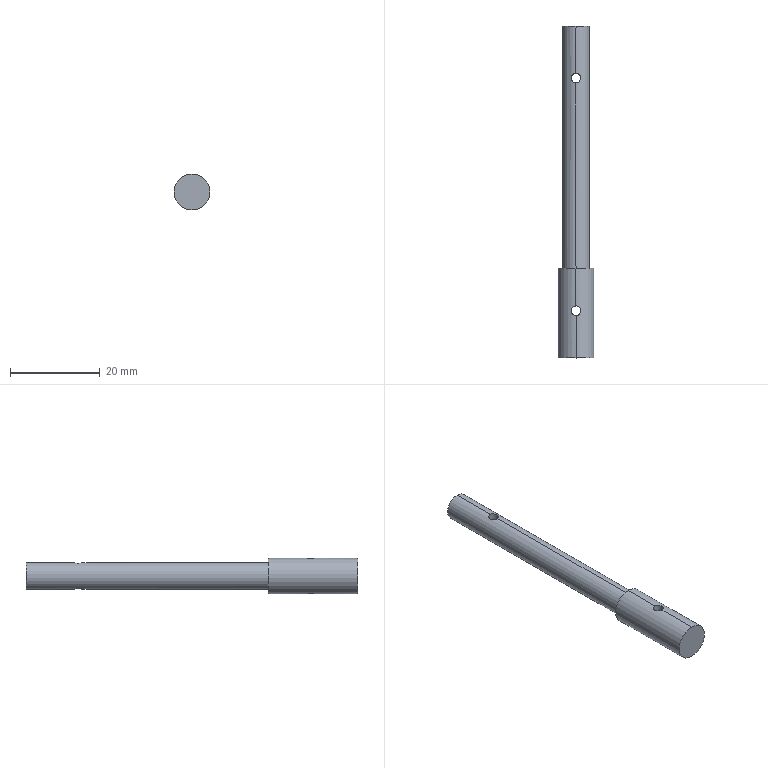Part | SolidWorks | features ICE 1, Revolution 1 | 1 solid | 11 faces | box 8 x 74 x 8 mm | volume 2480 mm3 | cylinder 8 | plane 3 | commonest cylinder face diameters 2.2 x4 6 x2 8 x2
STEP:
#1=CARTESIAN_POINT('',(0.,55.397,-3.));
#2=VERTEX_POINT('',#1);
#3=CARTESIAN_POINT('',(-1.1,56.497,-2.791));
#4=VERTEX_POINT('',#3);
#5=CARTESIAN_POINT('',(0.,55.397,-3.));
#6=CARTESIAN_POINT('',(-0.1445,55.397,-3.));
#7=CARTESIAN_POINT('',(-0.2902,55.427,-2.989));
#8=CARTESIAN_POINT('',(-0.556,55.537,-2.951));
#9=CARTESIAN_POINT('',(-0.6765,55.618,-2.925));
#10=CARTESIAN_POINT('',(-0.8798,55.822,-2.87));
#11=CARTESIAN_POINT('',(-0.9601,55.941,-2.843));
#12=CARTESIAN_POINT('',(-1.043,56.141,-2.813));
#13=CARTESIAN_POINT('',(-1.064,56.21,-2.805));
#14=CARTESIAN_POINT('',(-1.093,56.351,-2.794));
#15=CARTESIAN_POINT('',(-1.1,56.425,-2.791));
#16=CARTESIAN_POINT('',(-1.1,56.497,-2.791));
#17=B_SPLINE_CURVE_WITH_KNOTS('',3,(#5,#6,#7,#8,#9,#10,#11,#12,#13,#14,#15,#16),.UNSPECIFIED.,.F.,.F.,(4,2,2,2,2,4),(0.00347,0.003903,0.004337,0.00477,0.004987,0.005204),.UNSPECIFIED.);
#18=EDGE_CURVE('',#2,#4,#17,.T.);
#19=ORIENTED_EDGE('',*,*,#18,.T.);
#20=CARTESIAN_POINT('',(-1.1,56.497,2.791));
#21=VERTEX_POINT('',#20);
#22=CARTESIAN_POINT('',(-1.1,56.497,-15.));
#23=DIRECTION('',(0.,0.,1.));
#24=VECTOR('',#23,1000.);
#25=LINE('',#22,#24);
#26=EDGE_CURVE('',#4,#21,#25,.T.);
#27=ORIENTED_EDGE('',*,*,#26,.T.);
#28=CARTESIAN_POINT('',(0.,55.397,3.));
#29=VERTEX_POINT('',#28);
#30=CARTESIAN_POINT('',(-1.1,56.497,2.791));
#31=CARTESIAN_POINT('',(-1.1,56.353,2.791));
#32=CARTESIAN_POINT('',(-1.071,56.207,2.803));
#33=CARTESIAN_POINT('',(-0.9601,55.942,2.843));
#34=CARTESIAN_POINT('',(-0.8795,55.821,2.87));
#35=CARTESIAN_POINT('',(-0.6761,55.618,2.925));
#36=CARTESIAN_POINT('',(-0.5563,55.537,2.951));
#37=CARTESIAN_POINT('',(-0.3563,55.454,2.98));
#38=CARTESIAN_POINT('',(-0.2876,55.433,2.987));
#39=CARTESIAN_POINT('',(-0.1461,55.405,2.997));
#40=CARTESIAN_POINT('',(-0.07247,55.397,3.));
#41=CARTESIAN_POINT('',(0.,55.397,3.));
#42=B_SPLINE_CURVE_WITH_KNOTS('',3,(#30,#31,#32,#33,#34,#35,#36,#37,#38,#39,#40,#41),.UNSPECIFIED.,.F.,.F.,(4,2,2,2,2,4),(0.00347,0.003903,0.004336,0.00477,0.004987,0.005203),.UNSPECIFIED.);
#43=EDGE_CURVE('',#21,#29,#42,.T.);
#44=ORIENTED_EDGE('',*,*,#43,.T.);
#45=CARTESIAN_POINT('',(1.1,56.497,2.791));
#46=VERTEX_POINT('',#45);
#47=CARTESIAN_POINT('',(0.,55.397,3.));
#48=CARTESIAN_POINT('',(0.145,55.397,3.));
#49=CARTESIAN_POINT('',(0.2907,55.427,2.989));
#50=CARTESIAN_POINT('',(0.5558,55.537,2.951));
#51=CARTESIAN_POINT('',(0.6773,55.619,2.924));
#52=CARTESIAN_POINT('',(0.879,55.821,2.87));
#53=CARTESIAN_POINT('',(0.9599,55.941,2.843));
#54=CARTESIAN_POINT('',(1.071,56.208,2.803));
#55=CARTESIAN_POINT('',(1.1,56.351,2.791));
#56=CARTESIAN_POINT('',(1.1,56.497,2.791));
#57=B_SPLINE_CURVE_WITH_KNOTS('',3,(#47,#48,#49,#50,#51,#52,#53,#54,#55,#56),.UNSPECIFIED.,.F.,.F.,(4,2,2,2,4),(0.005203,0.005637,0.006071,0.006505,0.006938),.UNSPECIFIED.);
#58=EDGE_CURVE('',#29,#46,#57,.T.);
#59=ORIENTED_EDGE('',*,*,#58,.T.);
#60=CARTESIAN_POINT('',(1.1,56.497,-2.791));
#61=VERTEX_POINT('',#60);
#62=CARTESIAN_POINT('',(1.1,56.497,-15.));
#63=DIRECTION('',(0.,0.,1.));
#64=VECTOR('',#63,1000.);
#65=LINE('',#62,#64);
#66=EDGE_CURVE('',#61,#46,#65,.T.);
#67=ORIENTED_EDGE('',*,*,#66,.F.);
#68=CARTESIAN_POINT('',(1.1,56.497,-2.791));
#69=CARTESIAN_POINT('',(1.1,56.352,-2.791));
#70=CARTESIAN_POINT('',(1.071,56.208,-2.803));
#71=CARTESIAN_POINT('',(0.9594,55.94,-2.843));
#72=CARTESIAN_POINT('',(0.8783,55.82,-2.87));
#73=CARTESIAN_POINT('',(0.6763,55.618,-2.925));
#74=CARTESIAN_POINT('',(0.555,55.537,-2.951));
#75=CARTESIAN_POINT('',(0.2904,55.427,-2.989));
#76=CARTESIAN_POINT('',(0.1445,55.397,-3.));
#77=CARTESIAN_POINT('',(0.,55.397,-3.));
#78=B_SPLINE_CURVE_WITH_KNOTS('',3,(#68,#69,#70,#71,#72,#73,#74,#75,#76,#77),.UNSPECIFIED.,.F.,.F.,(4,2,2,2,4),(0.001735,0.002169,0.002603,0.003036,0.00347),.UNSPECIFIED.);
#79=EDGE_CURVE('',#61,#2,#78,.T.);
#80=ORIENTED_EDGE('',*,*,#79,.T.);
#81=EDGE_LOOP('',(#19,#27,#44,#59,#67,#80));
#82=FACE_OUTER_BOUND('',#81,.T.);
#83=CARTESIAN_POINT('',(0.,56.497,-15.));
#84=DIRECTION('',(0.,0.,1.));
#85=DIRECTION('',(1.,0.,0.));
#86=AXIS2_PLACEMENT_3D('',#83,#84,#85);
#87=CYLINDRICAL_SURFACE('',#86,1.1);
#88=ADVANCED_FACE('',(#82),#87,.F.);
#89=CARTESIAN_POINT('',(0.,3.497,-4.));
#90=VERTEX_POINT('',#89);
#91=CARTESIAN_POINT('',(-1.1,4.597,-3.846));
#92=VERTEX_POINT('',#91);
#93=CARTESIAN_POINT('',(0.,3.497,-4.));
#94=CARTESIAN_POINT('',(-0.144,3.497,-4.));
#95=CARTESIAN_POINT('',(-0.2894,3.526,-3.992));
#96=CARTESIAN_POINT('',(-0.5545,3.637,-3.964));
#97=CARTESIAN_POINT('',(-0.6762,3.718,-3.944));
#98=CARTESIAN_POINT('',(-0.8792,3.921,-3.904));
#99=CARTESIAN_POINT('',(-0.96,4.041,-3.884));
#100=CARTESIAN_POINT('',(-1.071,4.309,-3.854));
#101=CARTESIAN_POINT('',(-1.1,4.452,-3.846));
#102=CARTESIAN_POINT('',(-1.1,4.597,-3.846));
#103=B_SPLINE_CURVE_WITH_KNOTS('',3,(#93,#94,#95,#96,#97,#98,#99,#100,#101,#102),.UNSPECIFIED.,.F.,.F.,(4,2,2,2,4),(0.003456,0.003888,0.00432,0.004752,0.005183),.UNSPECIFIED.);
#104=EDGE_CURVE('',#90,#92,#103,.T.);
#105=ORIENTED_EDGE('',*,*,#104,.T.);
#106=CARTESIAN_POINT('',(-1.1,4.597,3.846));
#107=VERTEX_POINT('',#106);
#108=CARTESIAN_POINT('',(-1.1,4.597,-15.));
#109=DIRECTION('',(0.,0.,1.));
#110=VECTOR('',#109,1000.);
#111=LINE('',#108,#110);
#112=EDGE_CURVE('',#92,#107,#111,.T.);
#113=ORIENTED_EDGE('',*,*,#112,.T.);
#114=CARTESIAN_POINT('',(0.,3.497,4.));
#115=VERTEX_POINT('',#114);
#116=CARTESIAN_POINT('',(-1.1,4.597,3.846));
#117=CARTESIAN_POINT('',(-1.1,4.453,3.846));
#118=CARTESIAN_POINT('',(-1.071,4.308,3.854));
#119=CARTESIAN_POINT('',(-0.9608,4.043,3.883));
#120=CARTESIAN_POINT('',(-0.8795,3.921,3.903));
#121=CARTESIAN_POINT('',(-0.6766,3.718,3.944));
#122=CARTESIAN_POINT('',(-0.5564,3.637,3.963));
#123=CARTESIAN_POINT('',(-0.2883,3.526,3.992));
#124=CARTESIAN_POINT('',(-0.1451,3.497,4.));
#125=CARTESIAN_POINT('',(0.,3.497,4.));
#126=B_SPLINE_CURVE_WITH_KNOTS('',3,(#116,#117,#118,#119,#120,#121,#122,#123,#124,#125),.UNSPECIFIED.,.F.,.F.,(4,2,2,2,4),(0.003456,0.003888,0.00432,0.004752,0.005183),.UNSPECIFIED.);
#127=EDGE_CURVE('',#107,#115,#126,.T.);
#128=ORIENTED_EDGE('',*,*,#127,.T.);
#129=CARTESIAN_POINT('',(1.1,4.597,3.846));
#130=VERTEX_POINT('',#129);
#131=CARTESIAN_POINT('',(0.,3.497,4.));
#132=CARTESIAN_POINT('',(0.145,3.497,4.));
#133=CARTESIAN_POINT('',(0.2895,3.527,3.992));
#134=CARTESIAN_POINT('',(0.5547,3.637,3.964));
#135=CARTESIAN_POINT('',(0.6767,3.719,3.944));
#136=CARTESIAN_POINT('',(0.8785,3.92,3.904));
#137=CARTESIAN_POINT('',(0.9603,4.042,3.883));
#138=CARTESIAN_POINT('',(1.071,4.307,3.854));
#139=CARTESIAN_POINT('',(1.1,4.451,3.846));
#140=CARTESIAN_POINT('',(1.1,4.597,3.846));
#141=B_SPLINE_CURVE_WITH_KNOTS('',3,(#131,#132,#133,#134,#135,#136,#137,#138,#139,#140),.UNSPECIFIED.,.F.,.F.,(4,2,2,2,4),(0.005183,0.005615,0.006047,0.006479,0.006911),.UNSPECIFIED.);
#142=EDGE_CURVE('',#115,#130,#141,.T.);
#143=ORIENTED_EDGE('',*,*,#142,.T.);
#144=CARTESIAN_POINT('',(1.1,4.597,-3.846));
#145=VERTEX_POINT('',#144);
#146=CARTESIAN_POINT('',(1.1,4.597,-15.));
#147=DIRECTION('',(0.,0.,1.));
#148=VECTOR('',#147,1000.);
#149=LINE('',#146,#148);
#150=EDGE_CURVE('',#145,#130,#149,.T.);
#151=ORIENTED_EDGE('',*,*,#150,.F.);
#152=CARTESIAN_POINT('',(1.1,4.597,-3.846));
#153=CARTESIAN_POINT('',(1.1,4.453,-3.846));
#154=CARTESIAN_POINT('',(1.071,4.309,-3.854));
#155=CARTESIAN_POINT('',(0.9602,4.042,-3.883));
#156=CARTESIAN_POINT('',(0.8792,3.921,-3.904));
#157=CARTESIAN_POINT('',(0.6757,3.718,-3.944));
#158=CARTESIAN_POINT('',(0.5544,3.637,-3.964));
#159=CARTESIAN_POINT('',(0.2891,3.526,-3.992));
#160=CARTESIAN_POINT('',(0.144,3.497,-4.));
#161=CARTESIAN_POINT('',(0.,3.497,-4.));
#162=B_SPLINE_CURVE_WITH_KNOTS('',3,(#152,#153,#154,#155,#156,#157,#158,#159,#160,#161),.UNSPECIFIED.,.F.,.F.,(4,2,2,2,4),(0.001728,0.00216,0.002592,0.003024,0.003456),.UNSPECIFIED.);
#163=EDGE_CURVE('',#145,#90,#162,.T.);
#164=ORIENTED_EDGE('',*,*,#163,.T.);
#165=EDGE_LOOP('',(#105,#113,#128,#143,#151,#164));
#166=FACE_OUTER_BOUND('',#165,.T.);
#167=CARTESIAN_POINT('',(0.,4.597,-15.));
#168=DIRECTION('',(0.,0.,1.));
#169=DIRECTION('',(1.,0.,0.));
#170=AXIS2_PLACEMENT_3D('',#167,#168,#169);
#171=CYLINDRICAL_SURFACE('',#170,1.1);
#172=ADVANCED_FACE('',(#166),#171,.F.);
#173=CARTESIAN_POINT('',(0.,14.097,-4.));
#174=VERTEX_POINT('',#173);
#175=CARTESIAN_POINT('',(0.,14.097,4.));
#176=VERTEX_POINT('',#175);
#177=CARTESIAN_POINT('',(0.,14.097,0.));
#178=DIRECTION('',(0.,-1.,0.));
#179=DIRECTION('',(0.,0.,-1.));
#180=AXIS2_PLACEMENT_3D('',#177,#178,#179);
#181=CIRCLE('',#180,4.);
#182=EDGE_CURVE('',#174,#176,#181,.T.);
#183=ORIENTED_EDGE('',*,*,#182,.T.);
#184=CARTESIAN_POINT('',(0.,5.697,4.));
#185=VERTEX_POINT('',#184);
#186=CARTESIAN_POINT('',(0.,0.,4.));
#187=DIRECTION('',(0.,-1.,0.));
#188=VECTOR('',#187,1000.);
#189=LINE('',#186,#188);
#190=EDGE_CURVE('',#176,#185,#189,.T.);
#191=ORIENTED_EDGE('',*,*,#190,.T.);
#192=CARTESIAN_POINT('',(1.1,4.597,3.846));
#193=CARTESIAN_POINT('',(1.1,4.744,3.846));
#194=CARTESIAN_POINT('',(1.071,4.887,3.854));
#195=CARTESIAN_POINT('',(0.9602,5.153,3.883));
#196=CARTESIAN_POINT('',(0.8785,5.275,3.904));
#197=CARTESIAN_POINT('',(0.6765,5.476,3.944));
#198=CARTESIAN_POINT('',(0.5542,5.558,3.964));
#199=CARTESIAN_POINT('',(0.2896,5.668,3.992));
#200=CARTESIAN_POINT('',(0.1443,5.697,4.));
#201=CARTESIAN_POINT('',(0.,5.697,4.));
#202=B_SPLINE_CURVE_WITH_KNOTS('',3,(#192,#193,#194,#195,#196,#197,#198,#199,#200,#201),.UNSPECIFIED.,.F.,.F.,(4,2,2,2,4),(0.,0.0004321,0.0008642,0.001296,0.001728),.UNSPECIFIED.);
#203=EDGE_CURVE('',#130,#185,#202,.T.);
#204=ORIENTED_EDGE('',*,*,#203,.F.);
#205=ORIENTED_EDGE('',*,*,#142,.F.);
#206=CARTESIAN_POINT('',(0.,-5.903,4.));
#207=VERTEX_POINT('',#206);
#208=CARTESIAN_POINT('',(0.,0.,4.));
#209=DIRECTION('',(0.,-1.,0.));
#210=VECTOR('',#209,1000.);
#211=LINE('',#208,#210);
#212=EDGE_CURVE('',#115,#207,#211,.T.);
#213=ORIENTED_EDGE('',*,*,#212,.T.);
#214=CARTESIAN_POINT('',(0.,-5.903,-4.));
#215=VERTEX_POINT('',#214);
#216=CARTESIAN_POINT('',(0.,-5.903,0.));
#217=DIRECTION('',(0.,-1.,0.));
#218=DIRECTION('',(0.,0.,-1.));
#219=AXIS2_PLACEMENT_3D('',#216,#217,#218);
#220=CIRCLE('',#219,4.);
#221=EDGE_CURVE('',#215,#207,#220,.T.);
#222=ORIENTED_EDGE('',*,*,#221,.F.);
#223=CARTESIAN_POINT('',(0.,0.,-4.));
#224=DIRECTION('',(0.,-1.,0.));
#225=VECTOR('',#224,1000.);
#226=LINE('',#223,#225);
#227=EDGE_CURVE('',#90,#215,#226,.T.);
#228=ORIENTED_EDGE('',*,*,#227,.F.);
#229=ORIENTED_EDGE('',*,*,#163,.F.);
#230=CARTESIAN_POINT('',(0.,5.697,-4.));
#231=VERTEX_POINT('',#230);
#232=CARTESIAN_POINT('',(0.,5.697,-4.));
#233=CARTESIAN_POINT('',(0.1462,5.697,-4.));
#234=CARTESIAN_POINT('',(0.2895,5.668,-3.992));
#235=CARTESIAN_POINT('',(0.5557,5.558,-3.963));
#236=CARTESIAN_POINT('',(0.6773,5.476,-3.944));
#237=CARTESIAN_POINT('',(0.8792,5.274,-3.904));
#238=CARTESIAN_POINT('',(0.9609,5.152,-3.883));
#239=CARTESIAN_POINT('',(1.071,4.887,-3.854));
#240=CARTESIAN_POINT('',(1.1,4.742,-3.846));
#241=CARTESIAN_POINT('',(1.1,4.597,-3.846));
#242=B_SPLINE_CURVE_WITH_KNOTS('',3,(#232,#233,#234,#235,#236,#237,#238,#239,#240,#241),.UNSPECIFIED.,.F.,.F.,(4,2,2,2,4),(0.,0.0004321,0.0008642,0.001296,0.001728),.UNSPECIFIED.);
#243=EDGE_CURVE('',#231,#145,#242,.T.);
#244=ORIENTED_EDGE('',*,*,#243,.F.);
#245=CARTESIAN_POINT('',(0.,0.,-4.));
#246=DIRECTION('',(0.,-1.,0.));
#247=VECTOR('',#246,1000.);
#248=LINE('',#245,#247);
#249=EDGE_CURVE('',#174,#231,#248,.T.);
#250=ORIENTED_EDGE('',*,*,#249,.F.);
#251=EDGE_LOOP('',(#183,#191,#204,#205,#213,#222,#228,#229,#244,#250));
#252=FACE_OUTER_BOUND('',#251,.T.);
#253=CARTESIAN_POINT('',(0.,0.,0.));
#254=DIRECTION('',(0.,-1.,0.));
#255=DIRECTION('',(0.,0.,-1.));
#256=AXIS2_PLACEMENT_3D('',#253,#254,#255);
#257=CYLINDRICAL_SURFACE('',#256,4.);
#258=ADVANCED_FACE('',(#252),#257,.T.);
#259=CARTESIAN_POINT('',(0.,68.097,-3.));
#260=VERTEX_POINT('',#259);
#261=CARTESIAN_POINT('',(0.,68.097,3.));
#262=VERTEX_POINT('',#261);
#263=CARTESIAN_POINT('',(0.,68.097,0.));
#264=DIRECTION('',(0.,-1.,0.));
#265=DIRECTION('',(0.,0.,-1.));
#266=AXIS2_PLACEMENT_3D('',#263,#264,#265);
#267=CIRCLE('',#266,3.);
#268=EDGE_CURVE('',#260,#262,#267,.T.);
#269=ORIENTED_EDGE('',*,*,#268,.T.);
#270=CARTESIAN_POINT('',(0.,57.597,3.));
#271=VERTEX_POINT('',#270);
#272=CARTESIAN_POINT('',(0.,0.,3.));
#273=DIRECTION('',(0.,-1.,0.));
#274=VECTOR('',#273,1000.);
#275=LINE('',#272,#274);
#276=EDGE_CURVE('',#262,#271,#275,.T.);
#277=ORIENTED_EDGE('',*,*,#276,.T.);
#278=CARTESIAN_POINT('',(1.1,56.497,2.791));
#279=CARTESIAN_POINT('',(1.1,56.644,2.791));
#280=CARTESIAN_POINT('',(1.071,56.788,2.803));
#281=CARTESIAN_POINT('',(0.9597,57.054,2.843));
#282=CARTESIAN_POINT('',(0.8781,57.175,2.87));
#283=CARTESIAN_POINT('',(0.6769,57.376,2.924));
#284=CARTESIAN_POINT('',(0.5552,57.458,2.951));
#285=CARTESIAN_POINT('',(0.2907,57.568,2.989));
#286=CARTESIAN_POINT('',(0.145,57.597,3.));
#287=CARTESIAN_POINT('',(0.,57.597,3.));
#288=B_SPLINE_CURVE_WITH_KNOTS('',3,(#278,#279,#280,#281,#282,#283,#284,#285,#286,#287),.UNSPECIFIED.,.F.,.F.,(4,2,2,2,4),(0.,0.0004338,0.0008676,0.001301,0.001735),.UNSPECIFIED.);
#289=EDGE_CURVE('',#46,#271,#288,.T.);
#290=ORIENTED_EDGE('',*,*,#289,.F.);
#291=ORIENTED_EDGE('',*,*,#58,.F.);
#292=CARTESIAN_POINT('',(0.,14.097,3.));
#293=VERTEX_POINT('',#292);
#294=CARTESIAN_POINT('',(0.,0.,3.));
#295=DIRECTION('',(0.,-1.,0.));
#296=VECTOR('',#295,1000.);
#297=LINE('',#294,#296);
#298=EDGE_CURVE('',#29,#293,#297,.T.);
#299=ORIENTED_EDGE('',*,*,#298,.T.);
#300=CARTESIAN_POINT('',(0.,14.097,-3.));
#301=VERTEX_POINT('',#300);
#302=CARTESIAN_POINT('',(0.,14.097,0.));
#303=DIRECTION('',(0.,-1.,0.));
#304=DIRECTION('',(0.,0.,-1.));
#305=AXIS2_PLACEMENT_3D('',#302,#303,#304);
#306=CIRCLE('',#305,3.);
#307=EDGE_CURVE('',#301,#293,#306,.T.);
#308=ORIENTED_EDGE('',*,*,#307,.F.);
#309=CARTESIAN_POINT('',(0.,0.,-3.));
#310=DIRECTION('',(0.,-1.,0.));
#311=VECTOR('',#310,1000.);
#312=LINE('',#309,#311);
#313=EDGE_CURVE('',#2,#301,#312,.T.);
#314=ORIENTED_EDGE('',*,*,#313,.F.);
#315=ORIENTED_EDGE('',*,*,#79,.F.);
#316=CARTESIAN_POINT('',(0.,57.597,-3.));
#317=VERTEX_POINT('',#316);
#318=CARTESIAN_POINT('',(0.,57.597,-3.));
#319=CARTESIAN_POINT('',(0.1468,57.597,-3.));
#320=CARTESIAN_POINT('',(0.2907,57.568,-2.989));
#321=CARTESIAN_POINT('',(0.5567,57.457,-2.951));
#322=CARTESIAN_POINT('',(0.6779,57.375,-2.924));
#323=CARTESIAN_POINT('',(0.8789,57.174,-2.87));
#324=CARTESIAN_POINT('',(0.9605,57.052,-2.843));
#325=CARTESIAN_POINT('',(1.071,56.788,-2.803));
#326=CARTESIAN_POINT('',(1.1,56.642,-2.791));
#327=CARTESIAN_POINT('',(1.1,56.497,-2.791));
#328=B_SPLINE_CURVE_WITH_KNOTS('',3,(#318,#319,#320,#321,#322,#323,#324,#325,#326,#327),.UNSPECIFIED.,.F.,.F.,(4,2,2,2,4),(0.,0.0004339,0.0008677,0.001302,0.001735),.UNSPECIFIED.);
#329=EDGE_CURVE('',#317,#61,#328,.T.);
#330=ORIENTED_EDGE('',*,*,#329,.F.);
#331=CARTESIAN_POINT('',(0.,0.,-3.));
#332=DIRECTION('',(0.,-1.,0.));
#333=VECTOR('',#332,1000.);
#334=LINE('',#331,#333);
#335=EDGE_CURVE('',#260,#317,#334,.T.);
#336=ORIENTED_EDGE('',*,*,#335,.F.);
#337=EDGE_LOOP('',(#269,#277,#290,#291,#299,#308,#314,#315,#330,#336));
#338=FACE_OUTER_BOUND('',#337,.T.);
#339=CARTESIAN_POINT('',(0.,0.,0.));
#340=DIRECTION('',(0.,-1.,0.));
#341=DIRECTION('',(0.,0.,-1.));
#342=AXIS2_PLACEMENT_3D('',#339,#340,#341);
#343=CYLINDRICAL_SURFACE('',#342,3.);
#344=ADVANCED_FACE('',(#338),#343,.T.);
#345=ORIENTED_EDGE('',*,*,#268,.F.);
#346=CARTESIAN_POINT('',(0.,68.097,0.));
#347=DIRECTION('',(0.,-1.,0.));
#348=DIRECTION('',(0.,0.,-1.));
#349=AXIS2_PLACEMENT_3D('',#346,#347,#348);
#350=CIRCLE('',#349,3.);
#351=EDGE_CURVE('',#262,#260,#350,.T.);
#352=ORIENTED_EDGE('',*,*,#351,.F.);
#353=EDGE_LOOP('',(#345,#352));
#354=FACE_OUTER_BOUND('',#353,.T.);
#355=CARTESIAN_POINT('',(0.,68.097,0.));
#356=DIRECTION('',(0.,1.,0.));
#357=DIRECTION('',(0.,0.,1.));
#358=AXIS2_PLACEMENT_3D('',#355,#356,#357);
#359=PLANE('',#358);
#360=ADVANCED_FACE('',(#354),#359,.T.);
#361=ORIENTED_EDGE('',*,*,#276,.F.);
#362=ORIENTED_EDGE('',*,*,#351,.T.);
#363=ORIENTED_EDGE('',*,*,#335,.T.);
#364=CARTESIAN_POINT('',(-1.1,56.497,-2.791));
#365=CARTESIAN_POINT('',(-1.1,56.642,-2.791));
#366=CARTESIAN_POINT('',(-1.071,56.788,-2.803));
#367=CARTESIAN_POINT('',(-0.9602,57.053,-2.843));
#368=CARTESIAN_POINT('',(-0.8787,57.174,-2.87));
#369=CARTESIAN_POINT('',(-0.6769,57.376,-2.924));
#370=CARTESIAN_POINT('',(-0.5565,57.457,-2.951));
#371=CARTESIAN_POINT('',(-0.2896,57.568,-2.989));
#372=CARTESIAN_POINT('',(-0.1467,57.597,-3.));
#373=CARTESIAN_POINT('',(0.,57.597,-3.));
#374=B_SPLINE_CURVE_WITH_KNOTS('',3,(#364,#365,#366,#367,#368,#369,#370,#371,#372,#373),.UNSPECIFIED.,.F.,.F.,(4,2,2,2,4),(0.005204,0.005637,0.006071,0.006505,0.006939),.UNSPECIFIED.);
#375=EDGE_CURVE('',#4,#317,#374,.T.);
#376=ORIENTED_EDGE('',*,*,#375,.F.);
#377=ORIENTED_EDGE('',*,*,#18,.F.);
#378=ORIENTED_EDGE('',*,*,#313,.T.);
#379=CARTESIAN_POINT('',(0.,14.097,0.));
#380=DIRECTION('',(0.,-1.,0.));
#381=DIRECTION('',(0.,0.,-1.));
#382=AXIS2_PLACEMENT_3D('',#379,#380,#381);
#383=CIRCLE('',#382,3.);
#384=EDGE_CURVE('',#293,#301,#383,.T.);
#385=ORIENTED_EDGE('',*,*,#384,.F.);
#386=ORIENTED_EDGE('',*,*,#298,.F.);
#387=ORIENTED_EDGE('',*,*,#43,.F.);
#388=CARTESIAN_POINT('',(0.,57.597,3.));
#389=CARTESIAN_POINT('',(-0.145,57.597,3.));
#390=CARTESIAN_POINT('',(-0.2896,57.569,2.989));
#391=CARTESIAN_POINT('',(-0.5576,57.457,2.951));
#392=CARTESIAN_POINT('',(-0.6778,57.375,2.924));
#393=CARTESIAN_POINT('',(-0.8795,57.173,2.87));
#394=CARTESIAN_POINT('',(-0.9606,57.052,2.843));
#395=CARTESIAN_POINT('',(-1.071,56.788,2.803));
#396=CARTESIAN_POINT('',(-1.1,56.642,2.791));
#397=CARTESIAN_POINT('',(-1.1,56.497,2.791));
#398=B_SPLINE_CURVE_WITH_KNOTS('',3,(#388,#389,#390,#391,#392,#393,#394,#395,#396,#397),.UNSPECIFIED.,.F.,.F.,(4,2,2,2,4),(0.001735,0.002169,0.002602,0.003036,0.00347),.UNSPECIFIED.);
#399=EDGE_CURVE('',#271,#21,#398,.T.);
#400=ORIENTED_EDGE('',*,*,#399,.F.);
#401=EDGE_LOOP('',(#361,#362,#363,#376,#377,#378,#385,#386,#387,#400));
#402=FACE_OUTER_BOUND('',#401,.T.);
#403=CARTESIAN_POINT('',(0.,0.,0.));
#404=DIRECTION('',(0.,-1.,0.));
#405=DIRECTION('',(0.,0.,-1.));
#406=AXIS2_PLACEMENT_3D('',#403,#404,#405);
#407=CYLINDRICAL_SURFACE('',#406,3.);
#408=ADVANCED_FACE('',(#402),#407,.T.);
#409=ORIENTED_EDGE('',*,*,#307,.T.);
#410=ORIENTED_EDGE('',*,*,#384,.T.);
#411=EDGE_LOOP('',(#409,#410));
#412=FACE_BOUND('',#411,.T.);
#413=ORIENTED_EDGE('',*,*,#182,.F.);
#414=CARTESIAN_POINT('',(0.,14.097,0.));
#415=DIRECTION('',(0.,-1.,0.));
#416=DIRECTION('',(0.,0.,-1.));
#417=AXIS2_PLACEMENT_3D('',#414,#415,#416);
#418=CIRCLE('',#417,4.);
#419=EDGE_CURVE('',#176,#174,#418,.T.);
#420=ORIENTED_EDGE('',*,*,#419,.F.);
#421=EDGE_LOOP('',(#413,#420));
#422=FACE_OUTER_BOUND('',#421,.T.);
#423=CARTESIAN_POINT('',(3.,14.097,0.));
#424=DIRECTION('',(0.,1.,0.));
#425=DIRECTION('',(0.,0.,1.));
#426=AXIS2_PLACEMENT_3D('',#423,#424,#425);
#427=PLANE('',#426);
#428=ADVANCED_FACE('',(#412,#422),#427,.T.);
#429=ORIENTED_EDGE('',*,*,#190,.F.);
#430=ORIENTED_EDGE('',*,*,#419,.T.);
#431=ORIENTED_EDGE('',*,*,#249,.T.);
#432=CARTESIAN_POINT('',(-1.1,4.597,-3.846));
#433=CARTESIAN_POINT('',(-1.1,4.742,-3.846));
#434=CARTESIAN_POINT('',(-1.071,4.887,-3.854));
#435=CARTESIAN_POINT('',(-0.9607,5.152,-3.883));
#436=CARTESIAN_POINT('',(-0.879,5.274,-3.904));
#437=CARTESIAN_POINT('',(-0.6773,5.476,-3.944));
#438=CARTESIAN_POINT('',(-0.5555,5.558,-3.963));
#439=CARTESIAN_POINT('',(-0.2905,5.668,-3.992));
#440=CARTESIAN_POINT('',(-0.1461,5.697,-4.));
#441=CARTESIAN_POINT('',(0.,5.697,-4.));
#442=B_SPLINE_CURVE_WITH_KNOTS('',3,(#432,#433,#434,#435,#436,#437,#438,#439,#440,#441),.UNSPECIFIED.,.F.,.F.,(4,2,2,2,4),(0.005183,0.005615,0.006047,0.006479,0.006911),.UNSPECIFIED.);
#443=EDGE_CURVE('',#92,#231,#442,.T.);
#444=ORIENTED_EDGE('',*,*,#443,.F.);
#445=ORIENTED_EDGE('',*,*,#104,.F.);
#446=ORIENTED_EDGE('',*,*,#227,.T.);
#447=CARTESIAN_POINT('',(0.,-5.903,0.));
#448=DIRECTION('',(0.,-1.,0.));
#449=DIRECTION('',(0.,0.,-1.));
#450=AXIS2_PLACEMENT_3D('',#447,#448,#449);
#451=CIRCLE('',#450,4.);
#452=EDGE_CURVE('',#207,#215,#451,.T.);
#453=ORIENTED_EDGE('',*,*,#452,.F.);
#454=ORIENTED_EDGE('',*,*,#212,.F.);
#455=ORIENTED_EDGE('',*,*,#127,.F.);
#456=CARTESIAN_POINT('',(0.,5.697,4.));
#457=CARTESIAN_POINT('',(-0.1443,5.697,4.));
#458=CARTESIAN_POINT('',(-0.2887,5.669,3.992));
#459=CARTESIAN_POINT('',(-0.5559,5.558,3.963));
#460=CARTESIAN_POINT('',(-0.6767,5.477,3.944));
#461=CARTESIAN_POINT('',(-0.8799,5.273,3.903));
#462=CARTESIAN_POINT('',(-0.9609,5.152,3.883));
#463=CARTESIAN_POINT('',(-1.071,4.886,3.854));
#464=CARTESIAN_POINT('',(-1.1,4.741,3.846));
#465=CARTESIAN_POINT('',(-1.1,4.597,3.846));
#466=B_SPLINE_CURVE_WITH_KNOTS('',3,(#456,#457,#458,#459,#460,#461,#462,#463,#464,#465),.UNSPECIFIED.,.F.,.F.,(4,2,2,2,4),(0.001728,0.00216,0.002592,0.003024,0.003456),.UNSPECIFIED.);
#467=EDGE_CURVE('',#185,#107,#466,.T.);
#468=ORIENTED_EDGE('',*,*,#467,.F.);
#469=EDGE_LOOP('',(#429,#430,#431,#444,#445,#446,#453,#454,#455,#468));
#470=FACE_OUTER_BOUND('',#469,.T.);
#471=CARTESIAN_POINT('',(0.,0.,0.));
#472=DIRECTION('',(0.,-1.,0.));
#473=DIRECTION('',(0.,0.,-1.));
#474=AXIS2_PLACEMENT_3D('',#471,#472,#473);
#475=CYLINDRICAL_SURFACE('',#474,4.);
#476=ADVANCED_FACE('',(#470),#475,.T.);
#477=ORIENTED_EDGE('',*,*,#221,.T.);
#478=ORIENTED_EDGE('',*,*,#452,.T.);
#479=EDGE_LOOP('',(#477,#478));
#480=FACE_OUTER_BOUND('',#479,.T.);
#481=CARTESIAN_POINT('',(4.,-5.903,0.));
#482=DIRECTION('',(0.,-1.,0.));
#483=DIRECTION('',(0.,0.,-1.));
#484=AXIS2_PLACEMENT_3D('',#481,#482,#483);
#485=PLANE('',#484);
#486=ADVANCED_FACE('',(#480),#485,.T.);
#487=ORIENTED_EDGE('',*,*,#112,.F.);
#488=ORIENTED_EDGE('',*,*,#443,.T.);
#489=ORIENTED_EDGE('',*,*,#243,.T.);
#490=ORIENTED_EDGE('',*,*,#150,.T.);
#491=ORIENTED_EDGE('',*,*,#203,.T.);
#492=ORIENTED_EDGE('',*,*,#467,.T.);
#493=EDGE_LOOP('',(#487,#488,#489,#490,#491,#492));
#494=FACE_OUTER_BOUND('',#493,.T.);
#495=CARTESIAN_POINT('',(0.,4.597,-15.));
#496=DIRECTION('',(0.,0.,1.));
#497=DIRECTION('',(1.,0.,0.));
#498=AXIS2_PLACEMENT_3D('',#495,#496,#497);
#499=CYLINDRICAL_SURFACE('',#498,1.1);
#500=ADVANCED_FACE('',(#494),#499,.F.);
#501=ORIENTED_EDGE('',*,*,#26,.F.);
#502=ORIENTED_EDGE('',*,*,#375,.T.);
#503=ORIENTED_EDGE('',*,*,#329,.T.);
#504=ORIENTED_EDGE('',*,*,#66,.T.);
#505=ORIENTED_EDGE('',*,*,#289,.T.);
#506=ORIENTED_EDGE('',*,*,#399,.T.);
#507=EDGE_LOOP('',(#501,#502,#503,#504,#505,#506));
#508=FACE_OUTER_BOUND('',#507,.T.);
#509=CARTESIAN_POINT('',(0.,56.497,-15.));
#510=DIRECTION('',(0.,0.,1.));
#511=DIRECTION('',(1.,0.,0.));
#512=AXIS2_PLACEMENT_3D('',#509,#510,#511);
#513=CYLINDRICAL_SURFACE('',#512,1.1);
#514=ADVANCED_FACE('',(#508),#513,.F.);
#515=CLOSED_SHELL('',(#88,#172,#258,#344,#360,#408,#428,#476,#486,#500,#514));
#516=MANIFOLD_SOLID_BREP('',#515);
#517=CARTESIAN_POINT('',(0.,0.,0.));
#518=DIRECTION('',(0.,0.,1.));
#519=DIRECTION('',(1.,0.,0.));
#520=AXIS2_PLACEMENT_3D('',#517,#518,#519);
#521=(LENGTH_UNIT()NAMED_UNIT(*)SI_UNIT(.MILLI.,.METRE.));
#522=UNCERTAINTY_MEASURE_WITH_UNIT(LENGTH_MEASURE(0.00001),#521,'','');
#523=(NAMED_UNIT(*)PLANE_ANGLE_UNIT()SI_UNIT($,.RADIAN.));
#524=(NAMED_UNIT(*)SI_UNIT($,.STERADIAN.)SOLID_ANGLE_UNIT());
#525=(GEOMETRIC_REPRESENTATION_CONTEXT(3)GLOBAL_UNCERTAINTY_ASSIGNED_CONTEXT((#522))GLOBAL_UNIT_ASSIGNED_CONTEXT((#521,#523,#524))REPRESENTATION_CONTEXT('',''));
#526=ADVANCED_BREP_SHAPE_REPRESENTATION('',(#516,#520),#525);